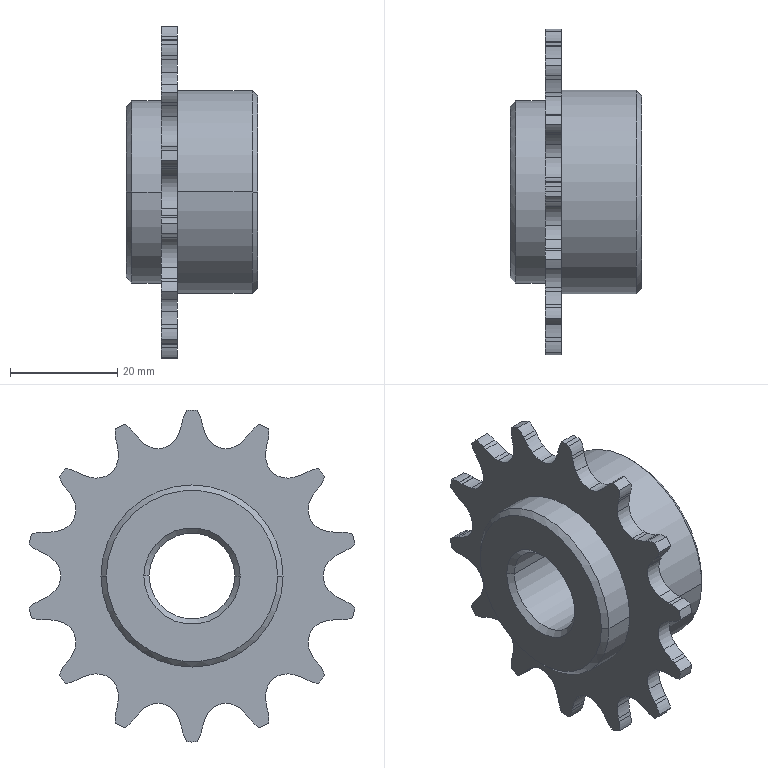Part | STEP file | 20305 | 1 solid | 148 faces | box 24.5 x 60.843 x 62 mm | volume 24740 mm3 | cylinder 108 | plane 32 | cone 8 | commonest cylinder face diameters 11.673 x32 20.732 x32 8.06 x22 62 x16 16 x2 34 x2